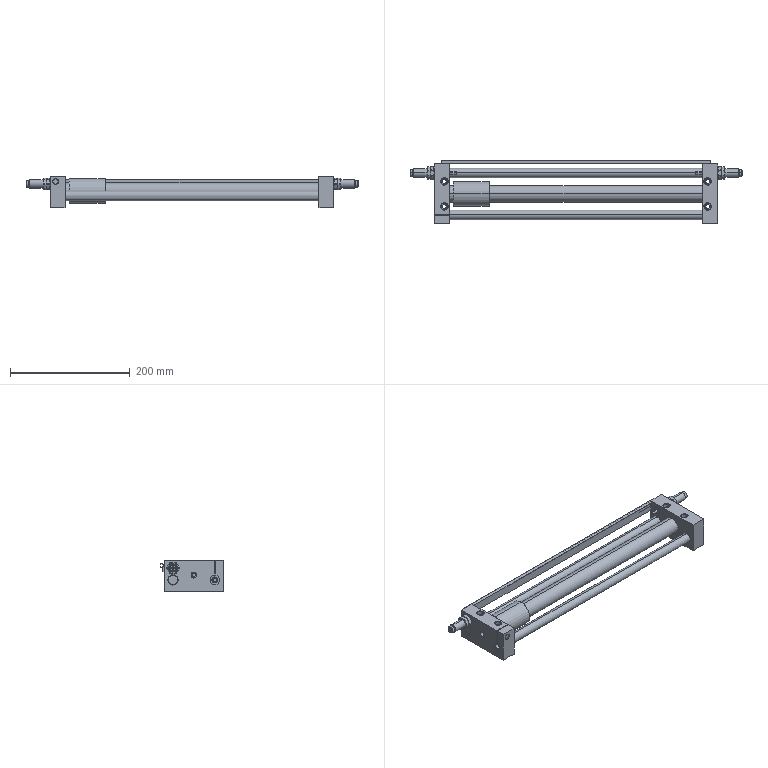Part | STEP file | _RMT-25X350-S-A(0)-GN-2_rod | 1 solid | 333 faces | box 555 x 106.4 x 53 mm | volume 757073 mm3 | cylinder 118 | plane 111 | cone 96 | spline 8 | commonest cylinder face diameters 20.5 x24 11 x12 16 x10 5 x8 6.647 x8 7 x8